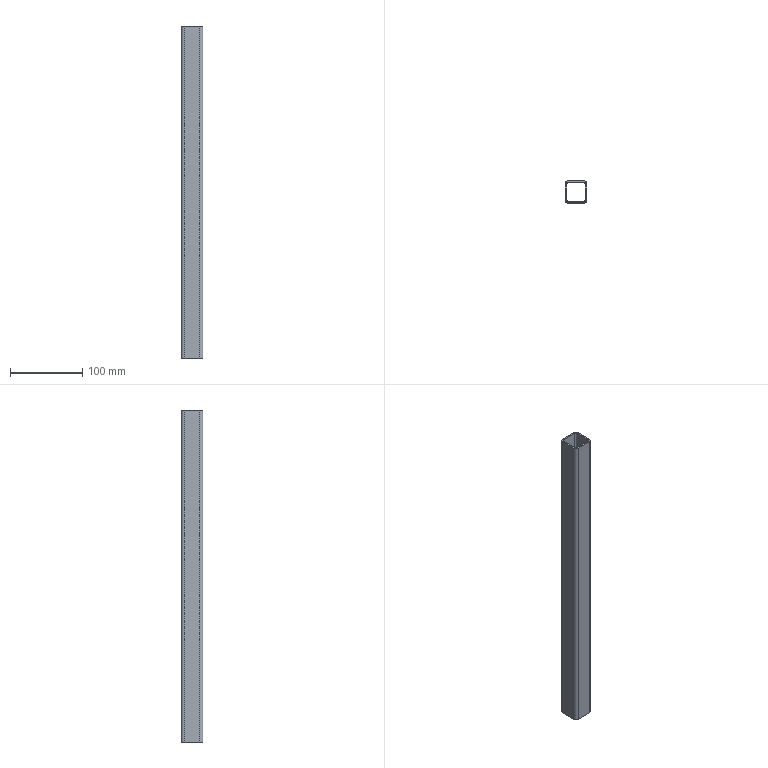Part | SolidWorks | features BaseBody 1 | 1 solid | 18 faces | box 30 x 30 x 460 mm | volume 98302 mm3 | plane 10 | cylinder 8 | commonest cylinder face diameters 4 x4 8 x4
STEP:
#1=CARTESIAN_POINT('',(-373.,-754.,-79.));
#2=VERTEX_POINT('',#1);
#3=CARTESIAN_POINT('',(-373.,-754.,381.));
#4=VERTEX_POINT('',#3);
#5=CARTESIAN_POINT('',(-373.,-754.,-109.));
#6=DIRECTION('',(0.,0.,1.));
#7=VECTOR('',#6,1000.);
#8=LINE('',#5,#7);
#9=EDGE_CURVE('',#2,#4,#8,.T.);
#10=ORIENTED_EDGE('',*,*,#9,.T.);
#11=CARTESIAN_POINT('',(-373.,-776.,381.));
#12=VERTEX_POINT('',#11);
#13=CARTESIAN_POINT('',(-373.,-754.,381.));
#14=DIRECTION('',(0.,-1.,0.));
#15=VECTOR('',#14,1000.);
#16=LINE('',#13,#15);
#17=EDGE_CURVE('',#4,#12,#16,.T.);
#18=ORIENTED_EDGE('',*,*,#17,.T.);
#19=CARTESIAN_POINT('',(-373.,-776.,-79.));
#20=VERTEX_POINT('',#19);
#21=CARTESIAN_POINT('',(-373.,-776.,-109.));
#22=DIRECTION('',(0.,0.,1.));
#23=VECTOR('',#22,1000.);
#24=LINE('',#21,#23);
#25=EDGE_CURVE('',#20,#12,#24,.T.);
#26=ORIENTED_EDGE('',*,*,#25,.F.);
#27=CARTESIAN_POINT('',(-373.,-754.,-79.));
#28=DIRECTION('',(0.,1.,0.));
#29=VECTOR('',#28,1000.);
#30=LINE('',#27,#29);
#31=EDGE_CURVE('',#20,#2,#30,.T.);
#32=ORIENTED_EDGE('',*,*,#31,.T.);
#33=EDGE_LOOP('',(#10,#18,#26,#32));
#34=FACE_OUTER_BOUND('',#33,.T.);
#35=CARTESIAN_POINT('',(-373.,-754.,-109.));
#36=DIRECTION('',(1.,0.,0.));
#37=DIRECTION('',(0.,0.,-1.));
#38=AXIS2_PLACEMENT_3D('',#35,#36,#37);
#39=PLANE('',#38);
#40=ADVANCED_FACE('',(#34),#39,.T.);
#41=CARTESIAN_POINT('',(-371.,-752.,-79.));
#42=VERTEX_POINT('',#41);
#43=CARTESIAN_POINT('',(-371.,-752.,381.));
#44=VERTEX_POINT('',#43);
#45=CARTESIAN_POINT('',(-371.,-752.,-109.));
#46=DIRECTION('',(0.,0.,1.));
#47=VECTOR('',#46,1000.);
#48=LINE('',#45,#47);
#49=EDGE_CURVE('',#42,#44,#48,.T.);
#50=ORIENTED_EDGE('',*,*,#49,.T.);
#51=CARTESIAN_POINT('',(-371.,-754.,381.));
#52=DIRECTION('',(0.,0.,1.));
#53=DIRECTION('',(1.,0.,0.));
#54=AXIS2_PLACEMENT_3D('',#51,#52,#53);
#55=CIRCLE('',#54,2.);
#56=EDGE_CURVE('',#44,#4,#55,.T.);
#57=ORIENTED_EDGE('',*,*,#56,.T.);
#58=ORIENTED_EDGE('',*,*,#9,.F.);
#59=CARTESIAN_POINT('',(-371.,-754.,-79.));
#60=DIRECTION('',(0.,0.,-1.));
#61=DIRECTION('',(-1.,0.,0.));
#62=AXIS2_PLACEMENT_3D('',#59,#60,#61);
#63=CIRCLE('',#62,2.);
#64=EDGE_CURVE('',#2,#42,#63,.T.);
#65=ORIENTED_EDGE('',*,*,#64,.T.);
#66=EDGE_LOOP('',(#50,#57,#58,#65));
#67=FACE_OUTER_BOUND('',#66,.T.);
#68=CARTESIAN_POINT('',(-371.,-754.,-109.));
#69=DIRECTION('',(0.,0.,1.));
#70=DIRECTION('',(1.,0.,0.));
#71=AXIS2_PLACEMENT_3D('',#68,#69,#70);
#72=CYLINDRICAL_SURFACE('',#71,2.);
#73=ADVANCED_FACE('',(#67),#72,.F.);
#74=CARTESIAN_POINT('',(-349.,-752.,-79.));
#75=VERTEX_POINT('',#74);
#76=CARTESIAN_POINT('',(-349.,-752.,381.));
#77=VERTEX_POINT('',#76);
#78=CARTESIAN_POINT('',(-349.,-752.,-109.));
#79=DIRECTION('',(0.,0.,1.));
#80=VECTOR('',#79,1000.);
#81=LINE('',#78,#80);
#82=EDGE_CURVE('',#75,#77,#81,.T.);
#83=ORIENTED_EDGE('',*,*,#82,.T.);
#84=CARTESIAN_POINT('',(-371.,-752.,381.));
#85=DIRECTION('',(-1.,0.,0.));
#86=VECTOR('',#85,1000.);
#87=LINE('',#84,#86);
#88=EDGE_CURVE('',#77,#44,#87,.T.);
#89=ORIENTED_EDGE('',*,*,#88,.T.);
#90=ORIENTED_EDGE('',*,*,#49,.F.);
#91=CARTESIAN_POINT('',(-371.,-752.,-79.));
#92=DIRECTION('',(1.,0.,0.));
#93=VECTOR('',#92,1000.);
#94=LINE('',#91,#93);
#95=EDGE_CURVE('',#42,#75,#94,.T.);
#96=ORIENTED_EDGE('',*,*,#95,.T.);
#97=EDGE_LOOP('',(#83,#89,#90,#96));
#98=FACE_OUTER_BOUND('',#97,.T.);
#99=CARTESIAN_POINT('',(-371.,-752.,-109.));
#100=DIRECTION('',(0.,-1.,0.));
#101=DIRECTION('',(0.,0.,-1.));
#102=AXIS2_PLACEMENT_3D('',#99,#100,#101);
#103=PLANE('',#102);
#104=ADVANCED_FACE('',(#98),#103,.T.);
#105=CARTESIAN_POINT('',(-347.,-754.,-79.));
#106=VERTEX_POINT('',#105);
#107=CARTESIAN_POINT('',(-347.,-754.,381.));
#108=VERTEX_POINT('',#107);
#109=CARTESIAN_POINT('',(-347.,-754.,-109.));
#110=DIRECTION('',(0.,0.,1.));
#111=VECTOR('',#110,1000.);
#112=LINE('',#109,#111);
#113=EDGE_CURVE('',#106,#108,#112,.T.);
#114=ORIENTED_EDGE('',*,*,#113,.T.);
#115=CARTESIAN_POINT('',(-349.,-754.,381.));
#116=DIRECTION('',(0.,0.,1.));
#117=DIRECTION('',(1.,0.,0.));
#118=AXIS2_PLACEMENT_3D('',#115,#116,#117);
#119=CIRCLE('',#118,2.);
#120=EDGE_CURVE('',#108,#77,#119,.T.);
#121=ORIENTED_EDGE('',*,*,#120,.T.);
#122=ORIENTED_EDGE('',*,*,#82,.F.);
#123=CARTESIAN_POINT('',(-349.,-754.,-79.));
#124=DIRECTION('',(0.,0.,-1.));
#125=DIRECTION('',(-1.,0.,0.));
#126=AXIS2_PLACEMENT_3D('',#123,#124,#125);
#127=CIRCLE('',#126,2.);
#128=EDGE_CURVE('',#75,#106,#127,.T.);
#129=ORIENTED_EDGE('',*,*,#128,.T.);
#130=EDGE_LOOP('',(#114,#121,#122,#129));
#131=FACE_OUTER_BOUND('',#130,.T.);
#132=CARTESIAN_POINT('',(-349.,-754.,-109.));
#133=DIRECTION('',(0.,0.,1.));
#134=DIRECTION('',(1.,0.,0.));
#135=AXIS2_PLACEMENT_3D('',#132,#133,#134);
#136=CYLINDRICAL_SURFACE('',#135,2.);
#137=ADVANCED_FACE('',(#131),#136,.F.);
#138=CARTESIAN_POINT('',(-347.,-776.,-79.));
#139=VERTEX_POINT('',#138);
#140=CARTESIAN_POINT('',(-347.,-776.,381.));
#141=VERTEX_POINT('',#140);
#142=CARTESIAN_POINT('',(-347.,-776.,-109.));
#143=DIRECTION('',(0.,0.,1.));
#144=VECTOR('',#143,1000.);
#145=LINE('',#142,#144);
#146=EDGE_CURVE('',#139,#141,#145,.T.);
#147=ORIENTED_EDGE('',*,*,#146,.T.);
#148=CARTESIAN_POINT('',(-347.,-776.,381.));
#149=DIRECTION('',(0.,1.,0.));
#150=VECTOR('',#149,1000.);
#151=LINE('',#148,#150);
#152=EDGE_CURVE('',#141,#108,#151,.T.);
#153=ORIENTED_EDGE('',*,*,#152,.T.);
#154=ORIENTED_EDGE('',*,*,#113,.F.);
#155=CARTESIAN_POINT('',(-347.,-776.,-79.));
#156=DIRECTION('',(0.,-1.,0.));
#157=VECTOR('',#156,1000.);
#158=LINE('',#155,#157);
#159=EDGE_CURVE('',#106,#139,#158,.T.);
#160=ORIENTED_EDGE('',*,*,#159,.T.);
#161=EDGE_LOOP('',(#147,#153,#154,#160));
#162=FACE_OUTER_BOUND('',#161,.T.);
#163=CARTESIAN_POINT('',(-347.,-776.,-109.));
#164=DIRECTION('',(-1.,0.,0.));
#165=DIRECTION('',(0.,0.,1.));
#166=AXIS2_PLACEMENT_3D('',#163,#164,#165);
#167=PLANE('',#166);
#168=ADVANCED_FACE('',(#162),#167,.T.);
#169=CARTESIAN_POINT('',(-349.,-778.,-79.));
#170=VERTEX_POINT('',#169);
#171=CARTESIAN_POINT('',(-349.,-778.,381.));
#172=VERTEX_POINT('',#171);
#173=CARTESIAN_POINT('',(-349.,-778.,-109.));
#174=DIRECTION('',(0.,0.,1.));
#175=VECTOR('',#174,1000.);
#176=LINE('',#173,#175);
#177=EDGE_CURVE('',#170,#172,#176,.T.);
#178=ORIENTED_EDGE('',*,*,#177,.T.);
#179=CARTESIAN_POINT('',(-349.,-776.,381.));
#180=DIRECTION('',(0.,0.,1.));
#181=DIRECTION('',(1.,0.,0.));
#182=AXIS2_PLACEMENT_3D('',#179,#180,#181);
#183=CIRCLE('',#182,2.);
#184=EDGE_CURVE('',#172,#141,#183,.T.);
#185=ORIENTED_EDGE('',*,*,#184,.T.);
#186=ORIENTED_EDGE('',*,*,#146,.F.);
#187=CARTESIAN_POINT('',(-349.,-776.,-79.));
#188=DIRECTION('',(0.,0.,-1.));
#189=DIRECTION('',(-1.,0.,0.));
#190=AXIS2_PLACEMENT_3D('',#187,#188,#189);
#191=CIRCLE('',#190,2.);
#192=EDGE_CURVE('',#139,#170,#191,.T.);
#193=ORIENTED_EDGE('',*,*,#192,.T.);
#194=EDGE_LOOP('',(#178,#185,#186,#193));
#195=FACE_OUTER_BOUND('',#194,.T.);
#196=CARTESIAN_POINT('',(-349.,-776.,-109.));
#197=DIRECTION('',(0.,0.,1.));
#198=DIRECTION('',(1.,0.,0.));
#199=AXIS2_PLACEMENT_3D('',#196,#197,#198);
#200=CYLINDRICAL_SURFACE('',#199,2.);
#201=ADVANCED_FACE('',(#195),#200,.F.);
#202=CARTESIAN_POINT('',(-371.,-778.,-79.));
#203=VERTEX_POINT('',#202);
#204=CARTESIAN_POINT('',(-371.,-778.,381.));
#205=VERTEX_POINT('',#204);
#206=CARTESIAN_POINT('',(-371.,-778.,-109.));
#207=DIRECTION('',(0.,0.,1.));
#208=VECTOR('',#207,1000.);
#209=LINE('',#206,#208);
#210=EDGE_CURVE('',#203,#205,#209,.T.);
#211=ORIENTED_EDGE('',*,*,#210,.T.);
#212=CARTESIAN_POINT('',(-349.,-778.,381.));
#213=DIRECTION('',(1.,0.,0.));
#214=VECTOR('',#213,1000.);
#215=LINE('',#212,#214);
#216=EDGE_CURVE('',#205,#172,#215,.T.);
#217=ORIENTED_EDGE('',*,*,#216,.T.);
#218=ORIENTED_EDGE('',*,*,#177,.F.);
#219=CARTESIAN_POINT('',(-349.,-778.,-79.));
#220=DIRECTION('',(-1.,0.,0.));
#221=VECTOR('',#220,1000.);
#222=LINE('',#219,#221);
#223=EDGE_CURVE('',#170,#203,#222,.T.);
#224=ORIENTED_EDGE('',*,*,#223,.T.);
#225=EDGE_LOOP('',(#211,#217,#218,#224));
#226=FACE_OUTER_BOUND('',#225,.T.);
#227=CARTESIAN_POINT('',(-349.,-778.,-109.));
#228=DIRECTION('',(0.,1.,0.));
#229=DIRECTION('',(0.,0.,1.));
#230=AXIS2_PLACEMENT_3D('',#227,#228,#229);
#231=PLANE('',#230);
#232=ADVANCED_FACE('',(#226),#231,.T.);
#233=ORIENTED_EDGE('',*,*,#25,.T.);
#234=CARTESIAN_POINT('',(-371.,-776.,381.));
#235=DIRECTION('',(0.,0.,1.));
#236=DIRECTION('',(1.,0.,0.));
#237=AXIS2_PLACEMENT_3D('',#234,#235,#236);
#238=CIRCLE('',#237,2.);
#239=EDGE_CURVE('',#12,#205,#238,.T.);
#240=ORIENTED_EDGE('',*,*,#239,.T.);
#241=ORIENTED_EDGE('',*,*,#210,.F.);
#242=CARTESIAN_POINT('',(-371.,-776.,-79.));
#243=DIRECTION('',(0.,0.,-1.));
#244=DIRECTION('',(-1.,0.,0.));
#245=AXIS2_PLACEMENT_3D('',#242,#243,#244);
#246=CIRCLE('',#245,2.);
#247=EDGE_CURVE('',#203,#20,#246,.T.);
#248=ORIENTED_EDGE('',*,*,#247,.T.);
#249=EDGE_LOOP('',(#233,#240,#241,#248));
#250=FACE_OUTER_BOUND('',#249,.T.);
#251=CARTESIAN_POINT('',(-371.,-776.,-109.));
#252=DIRECTION('',(0.,0.,1.));
#253=DIRECTION('',(1.,0.,0.));
#254=AXIS2_PLACEMENT_3D('',#251,#252,#253);
#255=CYLINDRICAL_SURFACE('',#254,2.);
#256=ADVANCED_FACE('',(#250),#255,.F.);
#257=ORIENTED_EDGE('',*,*,#223,.F.);
#258=ORIENTED_EDGE('',*,*,#192,.F.);
#259=ORIENTED_EDGE('',*,*,#159,.F.);
#260=ORIENTED_EDGE('',*,*,#128,.F.);
#261=ORIENTED_EDGE('',*,*,#95,.F.);
#262=ORIENTED_EDGE('',*,*,#64,.F.);
#263=ORIENTED_EDGE('',*,*,#31,.F.);
#264=ORIENTED_EDGE('',*,*,#247,.F.);
#265=EDGE_LOOP('',(#257,#258,#259,#260,#261,#262,#263,#264));
#266=FACE_BOUND('',#265,.T.);
#267=CARTESIAN_POINT('',(-371.,-780.,-79.));
#268=VERTEX_POINT('',#267);
#269=CARTESIAN_POINT('',(-375.,-776.,-79.));
#270=VERTEX_POINT('',#269);
#271=CARTESIAN_POINT('',(-371.,-776.,-79.));
#272=DIRECTION('',(0.,0.,-1.));
#273=DIRECTION('',(-1.,0.,0.));
#274=AXIS2_PLACEMENT_3D('',#271,#272,#273);
#275=CIRCLE('',#274,4.);
#276=EDGE_CURVE('',#268,#270,#275,.T.);
#277=ORIENTED_EDGE('',*,*,#276,.T.);
#278=CARTESIAN_POINT('',(-375.,-754.,-79.));
#279=VERTEX_POINT('',#278);
#280=CARTESIAN_POINT('',(-375.,-754.,-79.));
#281=DIRECTION('',(0.,1.,0.));
#282=VECTOR('',#281,1000.);
#283=LINE('',#280,#282);
#284=EDGE_CURVE('',#270,#279,#283,.T.);
#285=ORIENTED_EDGE('',*,*,#284,.T.);
#286=CARTESIAN_POINT('',(-371.,-750.,-79.));
#287=VERTEX_POINT('',#286);
#288=CARTESIAN_POINT('',(-371.,-754.,-79.));
#289=DIRECTION('',(0.,0.,-1.));
#290=DIRECTION('',(-1.,0.,0.));
#291=AXIS2_PLACEMENT_3D('',#288,#289,#290);
#292=CIRCLE('',#291,4.);
#293=EDGE_CURVE('',#279,#287,#292,.T.);
#294=ORIENTED_EDGE('',*,*,#293,.T.);
#295=CARTESIAN_POINT('',(-349.,-750.,-79.));
#296=VERTEX_POINT('',#295);
#297=CARTESIAN_POINT('',(375.,-750.,-79.));
#298=DIRECTION('',(-1.,0.,0.));
#299=VECTOR('',#298,1000.);
#300=LINE('',#297,#299);
#301=EDGE_CURVE('',#296,#287,#300,.T.);
#302=ORIENTED_EDGE('',*,*,#301,.F.);
#303=CARTESIAN_POINT('',(-345.,-754.,-79.));
#304=VERTEX_POINT('',#303);
#305=CARTESIAN_POINT('',(-349.,-754.,-79.));
#306=DIRECTION('',(0.,0.,-1.));
#307=DIRECTION('',(-1.,0.,0.));
#308=AXIS2_PLACEMENT_3D('',#305,#306,#307);
#309=CIRCLE('',#308,4.);
#310=EDGE_CURVE('',#296,#304,#309,.T.);
#311=ORIENTED_EDGE('',*,*,#310,.T.);
#312=CARTESIAN_POINT('',(-345.,-776.,-79.));
#313=VERTEX_POINT('',#312);
#314=CARTESIAN_POINT('',(-345.,-776.,-79.));
#315=DIRECTION('',(0.,-1.,0.));
#316=VECTOR('',#315,1000.);
#317=LINE('',#314,#316);
#318=EDGE_CURVE('',#304,#313,#317,.T.);
#319=ORIENTED_EDGE('',*,*,#318,.T.);
#320=CARTESIAN_POINT('',(-349.,-780.,-79.));
#321=VERTEX_POINT('',#320);
#322=CARTESIAN_POINT('',(-349.,-776.,-79.));
#323=DIRECTION('',(0.,0.,-1.));
#324=DIRECTION('',(-1.,0.,0.));
#325=AXIS2_PLACEMENT_3D('',#322,#323,#324);
#326=CIRCLE('',#325,4.);
#327=EDGE_CURVE('',#313,#321,#326,.T.);
#328=ORIENTED_EDGE('',*,*,#327,.T.);
#329=CARTESIAN_POINT('',(375.,-780.,-79.));
#330=DIRECTION('',(-1.,0.,0.));
#331=VECTOR('',#330,1000.);
#332=LINE('',#329,#331);
#333=EDGE_CURVE('',#321,#268,#332,.T.);
#334=ORIENTED_EDGE('',*,*,#333,.T.);
#335=EDGE_LOOP('',(#277,#285,#294,#302,#311,#319,#328,#334));
#336=FACE_OUTER_BOUND('',#335,.T.);
#337=CARTESIAN_POINT('',(375.,-776.,-79.));
#338=DIRECTION('',(0.,0.,-1.));
#339=DIRECTION('',(-1.,0.,0.));
#340=AXIS2_PLACEMENT_3D('',#337,#338,#339);
#341=PLANE('',#340);
#342=ADVANCED_FACE('',(#266,#336),#341,.T.);
#343=CARTESIAN_POINT('',(-345.,-776.,381.));
#344=VERTEX_POINT('',#343);
#345=CARTESIAN_POINT('',(-345.,-754.,381.));
#346=VERTEX_POINT('',#345);
#347=CARTESIAN_POINT('',(-345.,-776.,381.));
#348=DIRECTION('',(0.,1.,0.));
#349=VECTOR('',#348,1000.);
#350=LINE('',#347,#349);
#351=EDGE_CURVE('',#344,#346,#350,.T.);
#352=ORIENTED_EDGE('',*,*,#351,.F.);
#353=CARTESIAN_POINT('',(-345.,-776.,-109.));
#354=DIRECTION('',(0.,0.,1.));
#355=VECTOR('',#354,1000.);
#356=LINE('',#353,#355);
#357=EDGE_CURVE('',#313,#344,#356,.T.);
#358=ORIENTED_EDGE('',*,*,#357,.F.);
#359=ORIENTED_EDGE('',*,*,#318,.F.);
#360=CARTESIAN_POINT('',(-345.,-754.,-109.));
#361=DIRECTION('',(0.,0.,1.));
#362=VECTOR('',#361,1000.);
#363=LINE('',#360,#362);
#364=EDGE_CURVE('',#304,#346,#363,.T.);
#365=ORIENTED_EDGE('',*,*,#364,.T.);
#366=EDGE_LOOP('',(#352,#358,#359,#365));
#367=FACE_OUTER_BOUND('',#366,.T.);
#368=CARTESIAN_POINT('',(-345.,-776.,-109.));
#369=DIRECTION('',(-1.,0.,0.));
#370=DIRECTION('',(0.,0.,1.));
#371=AXIS2_PLACEMENT_3D('',#368,#369,#370);
#372=PLANE('',#371);
#373=ADVANCED_FACE('',(#367),#372,.F.);
#374=CARTESIAN_POINT('',(-349.,-750.,381.));
#375=VERTEX_POINT('',#374);
#376=CARTESIAN_POINT('',(-349.,-754.,381.));
#377=DIRECTION('',(0.,0.,1.));
#378=DIRECTION('',(1.,0.,0.));
#379=AXIS2_PLACEMENT_3D('',#376,#377,#378);
#380=CIRCLE('',#379,4.);
#381=EDGE_CURVE('',#346,#375,#380,.T.);
#382=ORIENTED_EDGE('',*,*,#381,.F.);
#383=ORIENTED_EDGE('',*,*,#364,.F.);
#384=ORIENTED_EDGE('',*,*,#310,.F.);
#385=CARTESIAN_POINT('',(-349.,-750.,-109.));
#386=DIRECTION('',(0.,0.,1.));
#387=VECTOR('',#386,1000.);
#388=LINE('',#385,#387);
#389=EDGE_CURVE('',#296,#375,#388,.T.);
#390=ORIENTED_EDGE('',*,*,#389,.T.);
#391=EDGE_LOOP('',(#382,#383,#384,#390));
#392=FACE_OUTER_BOUND('',#391,.T.);
#393=CARTESIAN_POINT('',(-349.,-754.,-109.));
#394=DIRECTION('',(0.,0.,1.));
#395=DIRECTION('',(1.,0.,0.));
#396=AXIS2_PLACEMENT_3D('',#393,#394,#395);
#397=CYLINDRICAL_SURFACE('',#396,4.);
#398=ADVANCED_FACE('',(#392),#397,.T.);
#399=CARTESIAN_POINT('',(-371.,-750.,381.));
#400=VERTEX_POINT('',#399);
#401=CARTESIAN_POINT('',(375.,-750.,381.));
#402=DIRECTION('',(-1.,0.,0.));
#403=VECTOR('',#402,1000.);
#404=LINE('',#401,#403);
#405=EDGE_CURVE('',#375,#400,#404,.T.);
#406=ORIENTED_EDGE('',*,*,#405,.F.);
#407=ORIENTED_EDGE('',*,*,#389,.F.);
#408=ORIENTED_EDGE('',*,*,#301,.T.);
#409=CARTESIAN_POINT('',(-371.,-750.,-109.));
#410=DIRECTION('',(0.,0.,1.));
#411=VECTOR('',#410,1000.);
#412=LINE('',#409,#411);
#413=EDGE_CURVE('',#287,#400,#412,.T.);
#414=ORIENTED_EDGE('',*,*,#413,.T.);
#415=EDGE_LOOP('',(#406,#407,#408,#414));
#416=FACE_OUTER_BOUND('',#415,.T.);
#417=CARTESIAN_POINT('',(-371.,-750.,-109.));
#418=DIRECTION('',(0.,-1.,0.));
#419=DIRECTION('',(0.,0.,-1.));
#420=AXIS2_PLACEMENT_3D('',#417,#418,#419);
#421=PLANE('',#420);
#422=ADVANCED_FACE('',(#416),#421,.F.);
#423=CARTESIAN_POINT('',(-375.,-754.,381.));
#424=VERTEX_POINT('',#423);
#425=CARTESIAN_POINT('',(-371.,-754.,381.));
#426=DIRECTION('',(0.,0.,1.));
#427=DIRECTION('',(1.,0.,0.));
#428=AXIS2_PLACEMENT_3D('',#425,#426,#427);
#429=CIRCLE('',#428,4.);
#430=EDGE_CURVE('',#400,#424,#429,.T.);
#431=ORIENTED_EDGE('',*,*,#430,.F.);
#432=ORIENTED_EDGE('',*,*,#413,.F.);
#433=ORIENTED_EDGE('',*,*,#293,.F.);
#434=CARTESIAN_POINT('',(-375.,-754.,-109.));
#435=DIRECTION('',(0.,0.,1.));
#436=VECTOR('',#435,1000.);
#437=LINE('',#434,#436);
#438=EDGE_CURVE('',#279,#424,#437,.T.);
#439=ORIENTED_EDGE('',*,*,#438,.T.);
#440=EDGE_LOOP('',(#431,#432,#433,#439));
#441=FACE_OUTER_BOUND('',#440,.T.);
#442=CARTESIAN_POINT('',(-371.,-754.,-109.));
#443=DIRECTION('',(0.,0.,1.));
#444=DIRECTION('',(1.,0.,0.));
#445=AXIS2_PLACEMENT_3D('',#442,#443,#444);
#446=CYLINDRICAL_SURFACE('',#445,4.);
#447=ADVANCED_FACE('',(#441),#446,.T.);
#448=CARTESIAN_POINT('',(-375.,-776.,381.));
#449=VERTEX_POINT('',#448);
#450=CARTESIAN_POINT('',(-375.,-754.,381.));
#451=DIRECTION('',(0.,-1.,0.));
#452=VECTOR('',#451,1000.);
#453=LINE('',#450,#452);
#454=EDGE_CURVE('',#424,#449,#453,.T.);
#455=ORIENTED_EDGE('',*,*,#454,.F.);
#456=ORIENTED_EDGE('',*,*,#438,.F.);
#457=ORIENTED_EDGE('',*,*,#284,.F.);
#458=CARTESIAN_POINT('',(-375.,-776.,-109.));
#459=DIRECTION('',(0.,0.,1.));
#460=VECTOR('',#459,1000.);
#461=LINE('',#458,#460);
#462=EDGE_CURVE('',#270,#449,#461,.T.);
#463=ORIENTED_EDGE('',*,*,#462,.T.);
#464=EDGE_LOOP('',(#455,#456,#457,#463));
#465=FACE_OUTER_BOUND('',#464,.T.);
#466=CARTESIAN_POINT('',(-375.,-754.,-109.));
#467=DIRECTION('',(1.,0.,0.));
#468=DIRECTION('',(0.,0.,-1.));
#469=AXIS2_PLACEMENT_3D('',#466,#467,#468);
#470=PLANE('',#469);
#471=ADVANCED_FACE('',(#465),#470,.F.);
#472=CARTESIAN_POINT('',(-371.,-780.,381.));
#473=VERTEX_POINT('',#472);
#474=CARTESIAN_POINT('',(-371.,-776.,381.));
#475=DIRECTION('',(0.,0.,1.));
#476=DIRECTION('',(1.,0.,0.));
#477=AXIS2_PLACEMENT_3D('',#474,#475,#476);
#478=CIRCLE('',#477,4.);
#479=EDGE_CURVE('',#449,#473,#478,.T.);
#480=ORIENTED_EDGE('',*,*,#479,.F.);
#481=ORIENTED_EDGE('',*,*,#462,.F.);
#482=ORIENTED_EDGE('',*,*,#276,.F.);
#483=CARTESIAN_POINT('',(-371.,-780.,-109.));
#484=DIRECTION('',(0.,0.,1.));
#485=VECTOR('',#484,1000.);
#486=LINE('',#483,#485);
#487=EDGE_CURVE('',#268,#473,#486,.T.);
#488=ORIENTED_EDGE('',*,*,#487,.T.);
#489=EDGE_LOOP('',(#480,#481,#482,#488));
#490=FACE_OUTER_BOUND('',#489,.T.);
#491=CARTESIAN_POINT('',(-371.,-776.,-109.));
#492=DIRECTION('',(0.,0.,1.));
#493=DIRECTION('',(1.,0.,0.));
#494=AXIS2_PLACEMENT_3D('',#491,#492,#493);
#495=CYLINDRICAL_SURFACE('',#494,4.);
#496=ADVANCED_FACE('',(#490),#495,.T.);
#497=CARTESIAN_POINT('',(-349.,-780.,381.));
#498=VERTEX_POINT('',#497);
#499=CARTESIAN_POINT('',(375.,-780.,381.));
#500=DIRECTION('',(-1.,0.,0.));
#501=VECTOR('',#500,1000.);
#502=LINE('',#499,#501);
#503=EDGE_CURVE('',#498,#473,#502,.T.);
#504=ORIENTED_EDGE('',*,*,#503,.T.);
#505=ORIENTED_EDGE('',*,*,#487,.F.);
#506=ORIENTED_EDGE('',*,*,#333,.F.);
#507=CARTESIAN_POINT('',(-349.,-780.,-109.));
#508=DIRECTION('',(0.,0.,1.));
#509=VECTOR('',#508,1000.);
#510=LINE('',#507,#509);
#511=EDGE_CURVE('',#321,#498,#510,.T.);
#512=ORIENTED_EDGE('',*,*,#511,.T.);
#513=EDGE_LOOP('',(#504,#505,#506,#512));
#514=FACE_OUTER_BOUND('',#513,.T.);
#515=CARTESIAN_POINT('',(-349.,-780.,-109.));
#516=DIRECTION('',(0.,1.,0.));
#517=DIRECTION('',(0.,0.,1.));
#518=AXIS2_PLACEMENT_3D('',#515,#516,#517);
#519=PLANE('',#518);
#520=ADVANCED_FACE('',(#514),#519,.F.);
#521=CARTESIAN_POINT('',(-349.,-776.,381.));
#522=DIRECTION('',(0.,0.,1.));
#523=DIRECTION('',(1.,0.,0.));
#524=AXIS2_PLACEMENT_3D('',#521,#522,#523);
#525=CIRCLE('',#524,4.);
#526=EDGE_CURVE('',#498,#344,#525,.T.);
#527=ORIENTED_EDGE('',*,*,#526,.F.);
#528=ORIENTED_EDGE('',*,*,#511,.F.);
#529=ORIENTED_EDGE('',*,*,#327,.F.);
#530=ORIENTED_EDGE('',*,*,#357,.T.);
#531=EDGE_LOOP('',(#527,#528,#529,#530));
#532=FACE_OUTER_BOUND('',#531,.T.);
#533=CARTESIAN_POINT('',(-349.,-776.,-109.));
#534=DIRECTION('',(0.,0.,1.));
#535=DIRECTION('',(1.,0.,0.));
#536=AXIS2_PLACEMENT_3D('',#533,#534,#535);
#537=CYLINDRICAL_SURFACE('',#536,4.);
#538=ADVANCED_FACE('',(#532),#537,.T.);
#539=ORIENTED_EDGE('',*,*,#17,.F.);
#540=ORIENTED_EDGE('',*,*,#56,.F.);
#541=ORIENTED_EDGE('',*,*,#88,.F.);
#542=ORIENTED_EDGE('',*,*,#120,.F.);
#543=ORIENTED_EDGE('',*,*,#152,.F.);
#544=ORIENTED_EDGE('',*,*,#184,.F.);
#545=ORIENTED_EDGE('',*,*,#216,.F.);
#546=ORIENTED_EDGE('',*,*,#239,.F.);
#547=EDGE_LOOP('',(#539,#540,#541,#542,#543,#544,#545,#546));
#548=FACE_BOUND('',#547,.T.);
#549=ORIENTED_EDGE('',*,*,#479,.T.);
#550=ORIENTED_EDGE('',*,*,#503,.F.);
#551=ORIENTED_EDGE('',*,*,#526,.T.);
#552=ORIENTED_EDGE('',*,*,#351,.T.);
#553=ORIENTED_EDGE('',*,*,#381,.T.);
#554=ORIENTED_EDGE('',*,*,#405,.T.);
#555=ORIENTED_EDGE('',*,*,#430,.T.);
#556=ORIENTED_EDGE('',*,*,#454,.T.);
#557=EDGE_LOOP('',(#549,#550,#551,#552,#553,#554,#555,#556));
#558=FACE_OUTER_BOUND('',#557,.T.);
#559=CARTESIAN_POINT('',(375.,-754.,381.));
#560=DIRECTION('',(0.,0.,1.));
#561=DIRECTION('',(1.,0.,0.));
#562=AXIS2_PLACEMENT_3D('',#559,#560,#561);
#563=PLANE('',#562);
#564=ADVANCED_FACE('',(#548,#558),#563,.T.);
#565=CLOSED_SHELL('',(#40,#73,#104,#137,#168,#201,#232,#256,#342,#373,#398,#422,#447,#471,#496,#520,#538,#564));
#566=MANIFOLD_SOLID_BREP('',#565);
#567=CARTESIAN_POINT('',(0.,0.,0.));
#568=DIRECTION('',(0.,0.,1.));
#569=DIRECTION('',(1.,0.,0.));
#570=AXIS2_PLACEMENT_3D('',#567,#568,#569);
#571=(LENGTH_UNIT()NAMED_UNIT(*)SI_UNIT(.MILLI.,.METRE.));
#572=UNCERTAINTY_MEASURE_WITH_UNIT(LENGTH_MEASURE(0.00001),#571,'','');
#573=(NAMED_UNIT(*)PLANE_ANGLE_UNIT()SI_UNIT($,.RADIAN.));
#574=(NAMED_UNIT(*)SI_UNIT($,.STERADIAN.)SOLID_ANGLE_UNIT());
#575=(GEOMETRIC_REPRESENTATION_CONTEXT(3)GLOBAL_UNCERTAINTY_ASSIGNED_CONTEXT((#572))GLOBAL_UNIT_ASSIGNED_CONTEXT((#571,#573,#574))REPRESENTATION_CONTEXT('',''));
#576=ADVANCED_BREP_SHAPE_REPRESENTATION('',(#566,#570),#575);